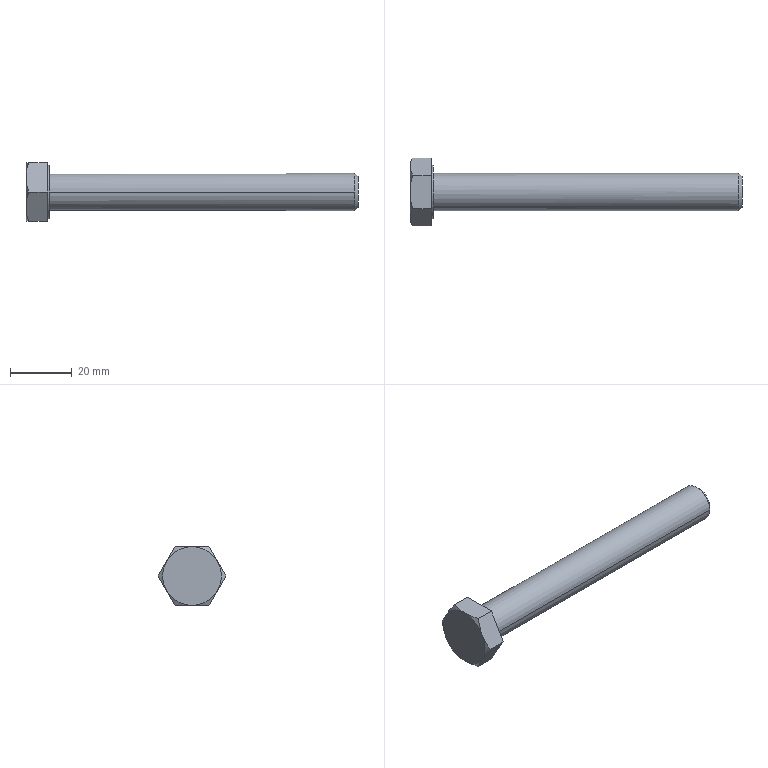Part | STEP file | DIN 931-1 - M12 x 100 | 1 solid | 22 faces | box 107.5 x 21.939 x 19 mm | volume 13582 mm3 | plane 10 | cone 8 | cylinder 4 | commonest cylinder face diameters 12 x2 17.4 x2